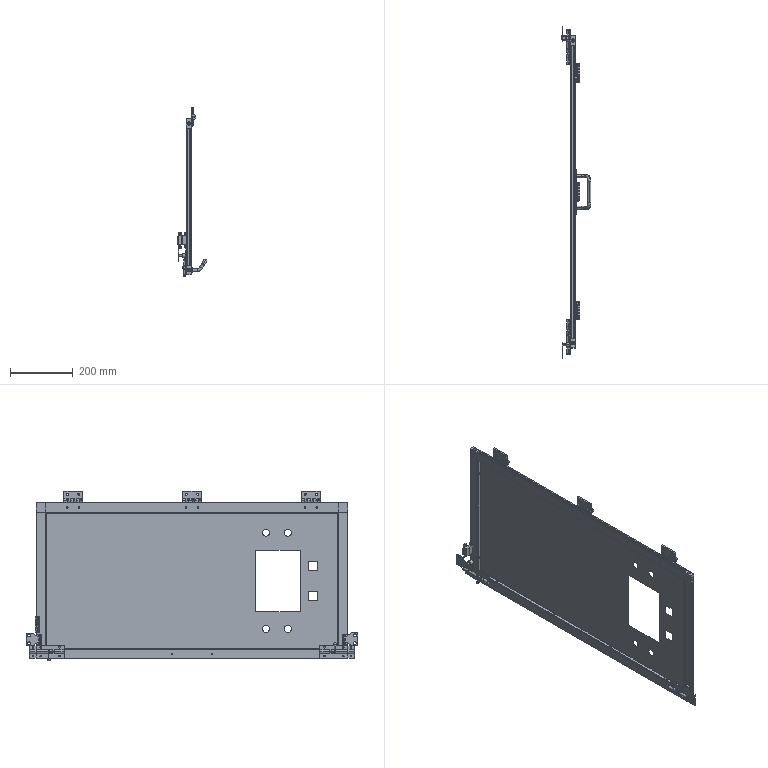Part | SolidWorks | 34 solids | 1110 faces | box 95.2 x 1060 x 541.75 mm | volume 1787457 mm3 | plane 632 | cylinder 418 | cone 48 | torus 6 | sphere 4 | spline 2 | commonest cylinder face diameters 5 x114 11 x56 7 x48 6.6 x24 14.5 x18 2.5 x16